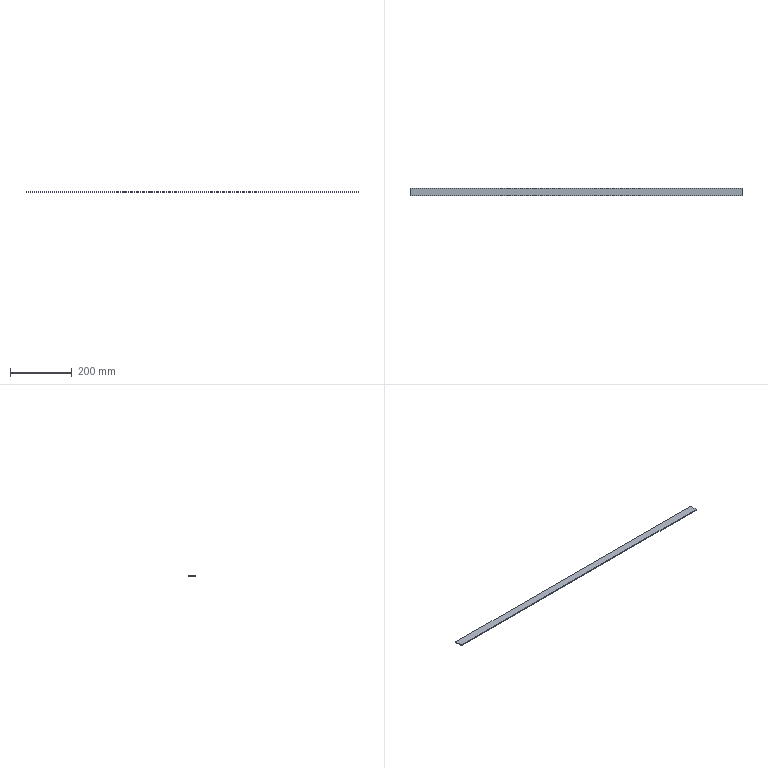Part | SolidWorks | features FlatPattern 1, SMBaseFlange 1, SheetMetal 1 | 1 solid | 6 faces | box 1072 x 25 x 3 mm | volume 80400 mm3 | plane 6
STEP:
#1=CARTESIAN_POINT('',(536.,-12.5,0.));
#2=VERTEX_POINT('',#1);
#3=CARTESIAN_POINT('',(536.,12.5,0.));
#4=VERTEX_POINT('',#3);
#5=CARTESIAN_POINT('',(536.,-12.5,0.));
#6=DIRECTION('',(0.,1.,0.));
#7=VECTOR('',#6,1000.);
#8=LINE('',#5,#7);
#9=EDGE_CURVE('',#2,#4,#8,.T.);
#10=ORIENTED_EDGE('',*,*,#9,.F.);
#11=CARTESIAN_POINT('',(536.,-12.5,-3.));
#12=VERTEX_POINT('',#11);
#13=CARTESIAN_POINT('',(536.,-12.5,-3.));
#14=DIRECTION('',(0.,0.,1.));
#15=VECTOR('',#14,1000.);
#16=LINE('',#13,#15);
#17=EDGE_CURVE('',#12,#2,#16,.T.);
#18=ORIENTED_EDGE('',*,*,#17,.F.);
#19=CARTESIAN_POINT('',(536.,12.5,-3.));
#20=VERTEX_POINT('',#19);
#21=CARTESIAN_POINT('',(536.,-12.5,-3.));
#22=DIRECTION('',(0.,1.,0.));
#23=VECTOR('',#22,1000.);
#24=LINE('',#21,#23);
#25=EDGE_CURVE('',#12,#20,#24,.T.);
#26=ORIENTED_EDGE('',*,*,#25,.T.);
#27=CARTESIAN_POINT('',(536.,12.5,-3.));
#28=DIRECTION('',(0.,0.,1.));
#29=VECTOR('',#28,1000.);
#30=LINE('',#27,#29);
#31=EDGE_CURVE('',#20,#4,#30,.T.);
#32=ORIENTED_EDGE('',*,*,#31,.T.);
#33=EDGE_LOOP('',(#10,#18,#26,#32));
#34=FACE_OUTER_BOUND('',#33,.T.);
#35=CARTESIAN_POINT('',(536.,-12.5,-3.));
#36=DIRECTION('',(1.,0.,0.));
#37=DIRECTION('',(0.,0.,-1.));
#38=AXIS2_PLACEMENT_3D('',#35,#36,#37);
#39=PLANE('',#38);
#40=ADVANCED_FACE('',(#34),#39,.T.);
#41=CARTESIAN_POINT('',(-536.,-12.5,0.));
#42=VERTEX_POINT('',#41);
#43=CARTESIAN_POINT('',(-536.,-12.5,0.));
#44=DIRECTION('',(1.,0.,0.));
#45=VECTOR('',#44,1000.);
#46=LINE('',#43,#45);
#47=EDGE_CURVE('',#42,#2,#46,.T.);
#48=ORIENTED_EDGE('',*,*,#47,.F.);
#49=CARTESIAN_POINT('',(-536.,-12.5,-3.));
#50=VERTEX_POINT('',#49);
#51=CARTESIAN_POINT('',(-536.,-12.5,-3.));
#52=DIRECTION('',(0.,0.,1.));
#53=VECTOR('',#52,1000.);
#54=LINE('',#51,#53);
#55=EDGE_CURVE('',#50,#42,#54,.T.);
#56=ORIENTED_EDGE('',*,*,#55,.F.);
#57=CARTESIAN_POINT('',(-536.,-12.5,-3.));
#58=DIRECTION('',(1.,0.,0.));
#59=VECTOR('',#58,1000.);
#60=LINE('',#57,#59);
#61=EDGE_CURVE('',#50,#12,#60,.T.);
#62=ORIENTED_EDGE('',*,*,#61,.T.);
#63=ORIENTED_EDGE('',*,*,#17,.T.);
#64=EDGE_LOOP('',(#48,#56,#62,#63));
#65=FACE_OUTER_BOUND('',#64,.T.);
#66=CARTESIAN_POINT('',(-536.,-12.5,-3.));
#67=DIRECTION('',(0.,-1.,0.));
#68=DIRECTION('',(0.,0.,-1.));
#69=AXIS2_PLACEMENT_3D('',#66,#67,#68);
#70=PLANE('',#69);
#71=ADVANCED_FACE('',(#65),#70,.T.);
#72=CARTESIAN_POINT('',(-536.,12.5,0.));
#73=VERTEX_POINT('',#72);
#74=CARTESIAN_POINT('',(-536.,-12.5,0.));
#75=DIRECTION('',(0.,-1.,0.));
#76=VECTOR('',#75,1000.);
#77=LINE('',#74,#76);
#78=EDGE_CURVE('',#73,#42,#77,.T.);
#79=ORIENTED_EDGE('',*,*,#78,.F.);
#80=CARTESIAN_POINT('',(-536.,12.5,-3.));
#81=VERTEX_POINT('',#80);
#82=CARTESIAN_POINT('',(-536.,12.5,-3.));
#83=DIRECTION('',(0.,0.,1.));
#84=VECTOR('',#83,1000.);
#85=LINE('',#82,#84);
#86=EDGE_CURVE('',#81,#73,#85,.T.);
#87=ORIENTED_EDGE('',*,*,#86,.F.);
#88=CARTESIAN_POINT('',(-536.,-12.5,-3.));
#89=DIRECTION('',(0.,-1.,0.));
#90=VECTOR('',#89,1000.);
#91=LINE('',#88,#90);
#92=EDGE_CURVE('',#81,#50,#91,.T.);
#93=ORIENTED_EDGE('',*,*,#92,.T.);
#94=ORIENTED_EDGE('',*,*,#55,.T.);
#95=EDGE_LOOP('',(#79,#87,#93,#94));
#96=FACE_OUTER_BOUND('',#95,.T.);
#97=CARTESIAN_POINT('',(-536.,-12.5,-3.));
#98=DIRECTION('',(-1.,0.,0.));
#99=DIRECTION('',(0.,0.,1.));
#100=AXIS2_PLACEMENT_3D('',#97,#98,#99);
#101=PLANE('',#100);
#102=ADVANCED_FACE('',(#96),#101,.T.);
#103=CARTESIAN_POINT('',(-536.,12.5,0.));
#104=DIRECTION('',(-1.,0.,0.));
#105=VECTOR('',#104,1000.);
#106=LINE('',#103,#105);
#107=EDGE_CURVE('',#4,#73,#106,.T.);
#108=ORIENTED_EDGE('',*,*,#107,.F.);
#109=ORIENTED_EDGE('',*,*,#31,.F.);
#110=CARTESIAN_POINT('',(-536.,12.5,-3.));
#111=DIRECTION('',(-1.,0.,0.));
#112=VECTOR('',#111,1000.);
#113=LINE('',#110,#112);
#114=EDGE_CURVE('',#20,#81,#113,.T.);
#115=ORIENTED_EDGE('',*,*,#114,.T.);
#116=ORIENTED_EDGE('',*,*,#86,.T.);
#117=EDGE_LOOP('',(#108,#109,#115,#116));
#118=FACE_OUTER_BOUND('',#117,.T.);
#119=CARTESIAN_POINT('',(-536.,12.5,-3.));
#120=DIRECTION('',(0.,1.,0.));
#121=DIRECTION('',(0.,0.,1.));
#122=AXIS2_PLACEMENT_3D('',#119,#120,#121);
#123=PLANE('',#122);
#124=ADVANCED_FACE('',(#118),#123,.T.);
#125=ORIENTED_EDGE('',*,*,#25,.F.);
#126=ORIENTED_EDGE('',*,*,#61,.F.);
#127=ORIENTED_EDGE('',*,*,#92,.F.);
#128=ORIENTED_EDGE('',*,*,#114,.F.);
#129=EDGE_LOOP('',(#125,#126,#127,#128));
#130=FACE_OUTER_BOUND('',#129,.T.);
#131=CARTESIAN_POINT('',(0.,0.,-3.));
#132=DIRECTION('',(0.,0.,-1.));
#133=DIRECTION('',(-1.,0.,0.));
#134=AXIS2_PLACEMENT_3D('',#131,#132,#133);
#135=PLANE('',#134);
#136=ADVANCED_FACE('',(#130),#135,.T.);
#137=ORIENTED_EDGE('',*,*,#9,.T.);
#138=ORIENTED_EDGE('',*,*,#107,.T.);
#139=ORIENTED_EDGE('',*,*,#78,.T.);
#140=ORIENTED_EDGE('',*,*,#47,.T.);
#141=EDGE_LOOP('',(#137,#138,#139,#140));
#142=FACE_OUTER_BOUND('',#141,.T.);
#143=CARTESIAN_POINT('',(0.,0.,0.));
#144=DIRECTION('',(0.,0.,-1.));
#145=DIRECTION('',(-1.,0.,0.));
#146=AXIS2_PLACEMENT_3D('',#143,#144,#145);
#147=PLANE('',#146);
#148=ADVANCED_FACE('',(#142),#147,.F.);
#149=CLOSED_SHELL('',(#40,#71,#102,#124,#136,#148));
#150=MANIFOLD_SOLID_BREP('',#149);
#151=CARTESIAN_POINT('',(0.,0.,0.));
#152=DIRECTION('',(0.,0.,1.));
#153=DIRECTION('',(1.,0.,0.));
#154=AXIS2_PLACEMENT_3D('',#151,#152,#153);
#155=(LENGTH_UNIT()NAMED_UNIT(*)SI_UNIT(.MILLI.,.METRE.));
#156=UNCERTAINTY_MEASURE_WITH_UNIT(LENGTH_MEASURE(0.00001),#155,'','');
#157=(NAMED_UNIT(*)PLANE_ANGLE_UNIT()SI_UNIT($,.RADIAN.));
#158=(NAMED_UNIT(*)SI_UNIT($,.STERADIAN.)SOLID_ANGLE_UNIT());
#159=(GEOMETRIC_REPRESENTATION_CONTEXT(3)GLOBAL_UNCERTAINTY_ASSIGNED_CONTEXT((#156))GLOBAL_UNIT_ASSIGNED_CONTEXT((#155,#157,#158))REPRESENTATION_CONTEXT('',''));
#160=ADVANCED_BREP_SHAPE_REPRESENTATION('',(#150,#154),#159);